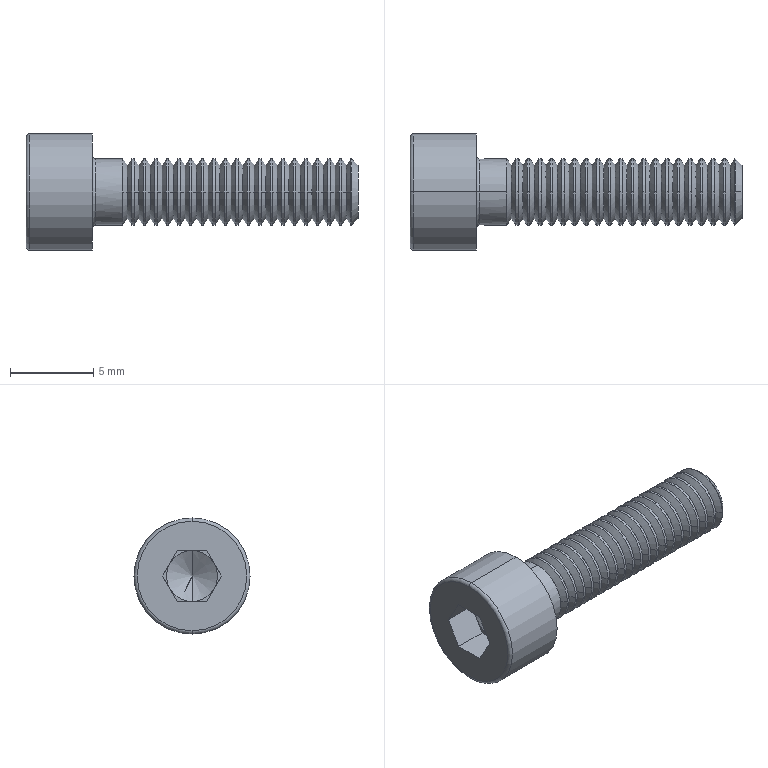Part | STEP file | Completa.sldasm-Part-63_Valor predeterminado | 1 solid | 147 faces | box 20 x 7 x 7 mm | volume 310.48 mm3 | cone 84 | cylinder 44 | plane 15 | torus 4 | commonest cylinder face diameters 4 x42 7 x2